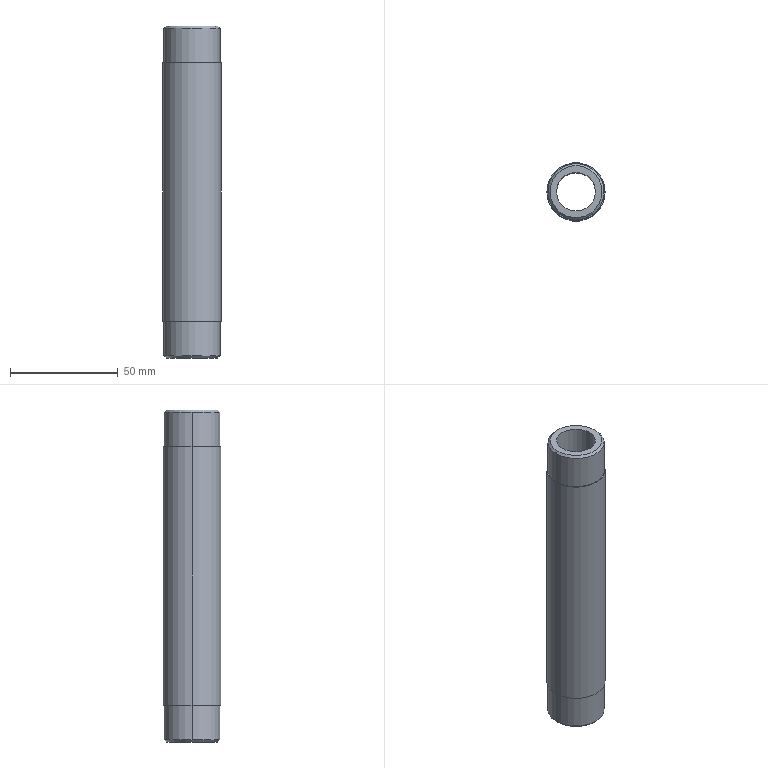Part | SolidWorks | features ICE 2, Chamfer 1, Extrusion 1, MirrorPattern 1 | 1 solid | 16 faces | box 27 x 27 x 154 mm | volume 47629 mm3 | cylinder 8 | cone 4 | plane 4 | commonest cylinder face diameters 26.1 x4 18 x2 27 x2
STEP:
#1=CARTESIAN_POINT('',(12.05,0.,77.));
#2=VERTEX_POINT('',#1);
#3=CARTESIAN_POINT('',(-12.05,0.,77.));
#4=VERTEX_POINT('',#3);
#5=CARTESIAN_POINT('',(0.,0.,77.));
#6=DIRECTION('',(0.,0.,1.));
#7=DIRECTION('',(1.,0.,0.));
#8=AXIS2_PLACEMENT_3D('',#5,#6,#7);
#9=CIRCLE('',#8,12.05);
#10=EDGE_CURVE('',#2,#4,#9,.T.);
#11=ORIENTED_EDGE('',*,*,#10,.F.);
#12=CARTESIAN_POINT('',(13.05,0.,76.));
#13=VERTEX_POINT('',#12);
#14=CARTESIAN_POINT('',(13.05,0.,76.));
#15=DIRECTION('',(0.7071,0.,-0.7071));
#16=VECTOR('',#15,1000.);
#17=LINE('',#14,#16);
#18=EDGE_CURVE('',#2,#13,#17,.T.);
#19=ORIENTED_EDGE('',*,*,#18,.T.);
#20=CARTESIAN_POINT('',(-13.05,0.,76.));
#21=VERTEX_POINT('',#20);
#22=CARTESIAN_POINT('',(0.,0.,76.));
#23=DIRECTION('',(0.,0.,-1.));
#24=DIRECTION('',(1.,0.,0.));
#25=AXIS2_PLACEMENT_3D('',#22,#23,#24);
#26=CIRCLE('',#25,13.05);
#27=EDGE_CURVE('',#21,#13,#26,.T.);
#28=ORIENTED_EDGE('',*,*,#27,.F.);
#29=CARTESIAN_POINT('',(-13.05,0.,76.));
#30=DIRECTION('',(-0.7071,0.,-0.7071));
#31=VECTOR('',#30,1000.);
#32=LINE('',#29,#31);
#33=EDGE_CURVE('',#4,#21,#32,.T.);
#34=ORIENTED_EDGE('',*,*,#33,.F.);
#35=EDGE_LOOP('',(#11,#19,#28,#34));
#36=FACE_OUTER_BOUND('',#35,.T.);
#37=CARTESIAN_POINT('',(0.,0.,76.));
#38=DIRECTION('',(0.,0.,-1.));
#39=DIRECTION('',(-1.,0.,0.));
#40=AXIS2_PLACEMENT_3D('',#37,#38,#39);
#41=CONICAL_SURFACE('',#40,13.05,0.7854);
#42=ADVANCED_FACE('',(#36),#41,.T.);
#43=CARTESIAN_POINT('',(-12.05,0.,-77.));
#44=VERTEX_POINT('',#43);
#45=CARTESIAN_POINT('',(12.05,0.,-77.));
#46=VERTEX_POINT('',#45);
#47=CARTESIAN_POINT('',(0.,0.,-77.));
#48=DIRECTION('',(0.,0.,-1.));
#49=DIRECTION('',(-1.,0.,0.));
#50=AXIS2_PLACEMENT_3D('',#47,#48,#49);
#51=CIRCLE('',#50,12.05);
#52=EDGE_CURVE('',#44,#46,#51,.T.);
#53=ORIENTED_EDGE('',*,*,#52,.F.);
#54=CARTESIAN_POINT('',(-13.05,0.,-76.));
#55=VERTEX_POINT('',#54);
#56=CARTESIAN_POINT('',(-12.05,0.,-77.));
#57=DIRECTION('',(-0.7071,0.,0.7071));
#58=VECTOR('',#57,1000.);
#59=LINE('',#56,#58);
#60=EDGE_CURVE('',#44,#55,#59,.T.);
#61=ORIENTED_EDGE('',*,*,#60,.T.);
#62=CARTESIAN_POINT('',(13.05,0.,-76.));
#63=VERTEX_POINT('',#62);
#64=CARTESIAN_POINT('',(0.,0.,-76.));
#65=DIRECTION('',(0.,0.,1.));
#66=DIRECTION('',(-1.,0.,0.));
#67=AXIS2_PLACEMENT_3D('',#64,#65,#66);
#68=CIRCLE('',#67,13.05);
#69=EDGE_CURVE('',#63,#55,#68,.T.);
#70=ORIENTED_EDGE('',*,*,#69,.F.);
#71=CARTESIAN_POINT('',(12.05,0.,-77.));
#72=DIRECTION('',(0.7071,0.,0.7071));
#73=VECTOR('',#72,1000.);
#74=LINE('',#71,#73);
#75=EDGE_CURVE('',#46,#63,#74,.T.);
#76=ORIENTED_EDGE('',*,*,#75,.F.);
#77=EDGE_LOOP('',(#53,#61,#70,#76));
#78=FACE_OUTER_BOUND('',#77,.T.);
#79=CARTESIAN_POINT('',(0.,0.,-77.));
#80=DIRECTION('',(0.,0.,1.));
#81=DIRECTION('',(1.,0.,0.));
#82=AXIS2_PLACEMENT_3D('',#79,#80,#81);
#83=CONICAL_SURFACE('',#82,12.05,0.7854);
#84=ADVANCED_FACE('',(#78),#83,.T.);
#85=CARTESIAN_POINT('',(9.,0.,77.));
#86=VERTEX_POINT('',#85);
#87=CARTESIAN_POINT('',(-9.,0.,77.));
#88=VERTEX_POINT('',#87);
#89=CARTESIAN_POINT('',(0.,0.,77.));
#90=DIRECTION('',(0.,0.,-1.));
#91=DIRECTION('',(1.,0.,0.));
#92=AXIS2_PLACEMENT_3D('',#89,#90,#91);
#93=CIRCLE('',#92,9.);
#94=EDGE_CURVE('',#86,#88,#93,.T.);
#95=ORIENTED_EDGE('',*,*,#94,.F.);
#96=CARTESIAN_POINT('',(9.,0.,-77.));
#97=VERTEX_POINT('',#96);
#98=CARTESIAN_POINT('',(9.,0.,77.001));
#99=DIRECTION('',(0.,0.,-1.));
#100=VECTOR('',#99,1000.);
#101=LINE('',#98,#100);
#102=EDGE_CURVE('',#86,#97,#101,.T.);
#103=ORIENTED_EDGE('',*,*,#102,.T.);
#104=CARTESIAN_POINT('',(-9.,0.,-77.));
#105=VERTEX_POINT('',#104);
#106=CARTESIAN_POINT('',(0.,0.,-77.));
#107=DIRECTION('',(0.,0.,-1.));
#108=DIRECTION('',(-1.,0.,0.));
#109=AXIS2_PLACEMENT_3D('',#106,#107,#108);
#110=CIRCLE('',#109,9.);
#111=EDGE_CURVE('',#97,#105,#110,.T.);
#112=ORIENTED_EDGE('',*,*,#111,.T.);
#113=CARTESIAN_POINT('',(-9.,0.,77.001));
#114=DIRECTION('',(0.,0.,-1.));
#115=VECTOR('',#114,1000.);
#116=LINE('',#113,#115);
#117=EDGE_CURVE('',#88,#105,#116,.T.);
#118=ORIENTED_EDGE('',*,*,#117,.F.);
#119=EDGE_LOOP('',(#95,#103,#112,#118));
#120=FACE_OUTER_BOUND('',#119,.T.);
#121=CARTESIAN_POINT('',(0.,0.,77.001));
#122=DIRECTION('',(0.,0.,-1.));
#123=DIRECTION('',(-1.,0.,0.));
#124=AXIS2_PLACEMENT_3D('',#121,#122,#123);
#125=CYLINDRICAL_SURFACE('',#124,9.);
#126=ADVANCED_FACE('',(#120),#125,.F.);
#127=ORIENTED_EDGE('',*,*,#27,.T.);
#128=CARTESIAN_POINT('',(13.05,0.,60.));
#129=VERTEX_POINT('',#128);
#130=CARTESIAN_POINT('',(13.05,0.,77.));
#131=DIRECTION('',(0.,0.,-1.));
#132=VECTOR('',#131,1000.);
#133=LINE('',#130,#132);
#134=EDGE_CURVE('',#13,#129,#133,.T.);
#135=ORIENTED_EDGE('',*,*,#134,.T.);
#136=CARTESIAN_POINT('',(-13.05,0.,60.));
#137=VERTEX_POINT('',#136);
#138=CARTESIAN_POINT('',(0.,0.,60.));
#139=DIRECTION('',(0.,0.,-1.));
#140=DIRECTION('',(-1.,0.,0.));
#141=AXIS2_PLACEMENT_3D('',#138,#139,#140);
#142=CIRCLE('',#141,13.05);
#143=EDGE_CURVE('',#137,#129,#142,.T.);
#144=ORIENTED_EDGE('',*,*,#143,.F.);
#145=CARTESIAN_POINT('',(-13.05,0.,77.));
#146=DIRECTION('',(0.,0.,-1.));
#147=VECTOR('',#146,1000.);
#148=LINE('',#145,#147);
#149=EDGE_CURVE('',#21,#137,#148,.T.);
#150=ORIENTED_EDGE('',*,*,#149,.F.);
#151=EDGE_LOOP('',(#127,#135,#144,#150));
#152=FACE_OUTER_BOUND('',#151,.T.);
#153=CARTESIAN_POINT('',(0.,0.,77.));
#154=DIRECTION('',(0.,0.,-1.));
#155=DIRECTION('',(-1.,0.,0.));
#156=AXIS2_PLACEMENT_3D('',#153,#154,#155);
#157=CYLINDRICAL_SURFACE('',#156,13.05);
#158=ADVANCED_FACE('',(#152),#157,.T.);
#159=ORIENTED_EDGE('',*,*,#69,.T.);
#160=CARTESIAN_POINT('',(-13.05,0.,-60.));
#161=VERTEX_POINT('',#160);
#162=CARTESIAN_POINT('',(-13.05,0.,-77.));
#163=DIRECTION('',(0.,0.,1.));
#164=VECTOR('',#163,1000.);
#165=LINE('',#162,#164);
#166=EDGE_CURVE('',#55,#161,#165,.T.);
#167=ORIENTED_EDGE('',*,*,#166,.T.);
#168=CARTESIAN_POINT('',(13.05,0.,-60.));
#169=VERTEX_POINT('',#168);
#170=CARTESIAN_POINT('',(0.,0.,-60.));
#171=DIRECTION('',(0.,0.,-1.));
#172=DIRECTION('',(-1.,0.,0.));
#173=AXIS2_PLACEMENT_3D('',#170,#171,#172);
#174=CIRCLE('',#173,13.05);
#175=EDGE_CURVE('',#161,#169,#174,.T.);
#176=ORIENTED_EDGE('',*,*,#175,.T.);
#177=CARTESIAN_POINT('',(13.05,0.,-77.));
#178=DIRECTION('',(0.,0.,1.));
#179=VECTOR('',#178,1000.);
#180=LINE('',#177,#179);
#181=EDGE_CURVE('',#63,#169,#180,.T.);
#182=ORIENTED_EDGE('',*,*,#181,.F.);
#183=EDGE_LOOP('',(#159,#167,#176,#182));
#184=FACE_OUTER_BOUND('',#183,.T.);
#185=CARTESIAN_POINT('',(0.,0.,-77.));
#186=DIRECTION('',(0.,0.,1.));
#187=DIRECTION('',(1.,0.,0.));
#188=AXIS2_PLACEMENT_3D('',#185,#186,#187);
#189=CYLINDRICAL_SURFACE('',#188,13.05);
#190=ADVANCED_FACE('',(#184),#189,.T.);
#191=CARTESIAN_POINT('',(13.5,0.,60.));
#192=VERTEX_POINT('',#191);
#193=CARTESIAN_POINT('',(-13.5,0.,60.));
#194=VERTEX_POINT('',#193);
#195=CARTESIAN_POINT('',(0.,0.,60.));
#196=DIRECTION('',(0.,0.,1.));
#197=DIRECTION('',(1.,0.,0.));
#198=AXIS2_PLACEMENT_3D('',#195,#196,#197);
#199=CIRCLE('',#198,13.5);
#200=EDGE_CURVE('',#192,#194,#199,.T.);
#201=ORIENTED_EDGE('',*,*,#200,.F.);
#202=CARTESIAN_POINT('',(13.5,0.,-60.));
#203=VERTEX_POINT('',#202);
#204=CARTESIAN_POINT('',(13.5,0.,60.));
#205=DIRECTION('',(0.,0.,-1.));
#206=VECTOR('',#205,1000.);
#207=LINE('',#204,#206);
#208=EDGE_CURVE('',#192,#203,#207,.T.);
#209=ORIENTED_EDGE('',*,*,#208,.T.);
#210=CARTESIAN_POINT('',(-13.5,0.,-60.));
#211=VERTEX_POINT('',#210);
#212=CARTESIAN_POINT('',(0.,0.,-60.));
#213=DIRECTION('',(0.,0.,1.));
#214=DIRECTION('',(1.,0.,0.));
#215=AXIS2_PLACEMENT_3D('',#212,#213,#214);
#216=CIRCLE('',#215,13.5);
#217=EDGE_CURVE('',#203,#211,#216,.T.);
#218=ORIENTED_EDGE('',*,*,#217,.T.);
#219=CARTESIAN_POINT('',(-13.5,0.,60.));
#220=DIRECTION('',(0.,0.,-1.));
#221=VECTOR('',#220,1000.);
#222=LINE('',#219,#221);
#223=EDGE_CURVE('',#194,#211,#222,.T.);
#224=ORIENTED_EDGE('',*,*,#223,.F.);
#225=EDGE_LOOP('',(#201,#209,#218,#224));
#226=FACE_OUTER_BOUND('',#225,.T.);
#227=CARTESIAN_POINT('',(0.,0.,60.));
#228=DIRECTION('',(0.,0.,-1.));
#229=DIRECTION('',(-1.,0.,0.));
#230=AXIS2_PLACEMENT_3D('',#227,#228,#229);
#231=CYLINDRICAL_SURFACE('',#230,13.5);
#232=ADVANCED_FACE('',(#226),#231,.T.);
#233=ORIENTED_EDGE('',*,*,#208,.F.);
#234=CARTESIAN_POINT('',(0.,0.,60.));
#235=DIRECTION('',(0.,0.,1.));
#236=DIRECTION('',(1.,0.,0.));
#237=AXIS2_PLACEMENT_3D('',#234,#235,#236);
#238=CIRCLE('',#237,13.5);
#239=EDGE_CURVE('',#194,#192,#238,.T.);
#240=ORIENTED_EDGE('',*,*,#239,.F.);
#241=ORIENTED_EDGE('',*,*,#223,.T.);
#242=CARTESIAN_POINT('',(0.,0.,-60.));
#243=DIRECTION('',(0.,0.,1.));
#244=DIRECTION('',(1.,0.,0.));
#245=AXIS2_PLACEMENT_3D('',#242,#243,#244);
#246=CIRCLE('',#245,13.5);
#247=EDGE_CURVE('',#211,#203,#246,.T.);
#248=ORIENTED_EDGE('',*,*,#247,.T.);
#249=EDGE_LOOP('',(#233,#240,#241,#248));
#250=FACE_OUTER_BOUND('',#249,.T.);
#251=CARTESIAN_POINT('',(0.,0.,60.));
#252=DIRECTION('',(0.,0.,-1.));
#253=DIRECTION('',(-1.,0.,0.));
#254=AXIS2_PLACEMENT_3D('',#251,#252,#253);
#255=CYLINDRICAL_SURFACE('',#254,13.5);
#256=ADVANCED_FACE('',(#250),#255,.T.);
#257=ORIENTED_EDGE('',*,*,#143,.T.);
#258=CARTESIAN_POINT('',(0.,0.,60.));
#259=DIRECTION('',(0.,0.,-1.));
#260=DIRECTION('',(-1.,0.,0.));
#261=AXIS2_PLACEMENT_3D('',#258,#259,#260);
#262=CIRCLE('',#261,13.05);
#263=EDGE_CURVE('',#129,#137,#262,.T.);
#264=ORIENTED_EDGE('',*,*,#263,.T.);
#265=EDGE_LOOP('',(#257,#264));
#266=FACE_BOUND('',#265,.T.);
#267=ORIENTED_EDGE('',*,*,#239,.T.);
#268=ORIENTED_EDGE('',*,*,#200,.T.);
#269=EDGE_LOOP('',(#267,#268));
#270=FACE_OUTER_BOUND('',#269,.T.);
#271=CARTESIAN_POINT('',(0.,0.,60.));
#272=DIRECTION('',(0.,0.,1.));
#273=DIRECTION('',(1.,0.,0.));
#274=AXIS2_PLACEMENT_3D('',#271,#272,#273);
#275=PLANE('',#274);
#276=ADVANCED_FACE('',(#266,#270),#275,.T.);
#277=CARTESIAN_POINT('',(0.,0.,-60.));
#278=DIRECTION('',(0.,0.,-1.));
#279=DIRECTION('',(-1.,0.,0.));
#280=AXIS2_PLACEMENT_3D('',#277,#278,#279);
#281=CIRCLE('',#280,13.05);
#282=EDGE_CURVE('',#169,#161,#281,.T.);
#283=ORIENTED_EDGE('',*,*,#282,.F.);
#284=ORIENTED_EDGE('',*,*,#175,.F.);
#285=EDGE_LOOP('',(#283,#284));
#286=FACE_BOUND('',#285,.T.);
#287=ORIENTED_EDGE('',*,*,#247,.F.);
#288=ORIENTED_EDGE('',*,*,#217,.F.);
#289=EDGE_LOOP('',(#287,#288));
#290=FACE_OUTER_BOUND('',#289,.T.);
#291=CARTESIAN_POINT('',(0.,0.,-60.));
#292=DIRECTION('',(0.,0.,1.));
#293=DIRECTION('',(1.,0.,0.));
#294=AXIS2_PLACEMENT_3D('',#291,#292,#293);
#295=PLANE('',#294);
#296=ADVANCED_FACE('',(#286,#290),#295,.F.);
#297=ORIENTED_EDGE('',*,*,#166,.F.);
#298=CARTESIAN_POINT('',(0.,0.,-76.));
#299=DIRECTION('',(0.,0.,1.));
#300=DIRECTION('',(-1.,0.,0.));
#301=AXIS2_PLACEMENT_3D('',#298,#299,#300);
#302=CIRCLE('',#301,13.05);
#303=EDGE_CURVE('',#55,#63,#302,.T.);
#304=ORIENTED_EDGE('',*,*,#303,.T.);
#305=ORIENTED_EDGE('',*,*,#181,.T.);
#306=ORIENTED_EDGE('',*,*,#282,.T.);
#307=EDGE_LOOP('',(#297,#304,#305,#306));
#308=FACE_OUTER_BOUND('',#307,.T.);
#309=CARTESIAN_POINT('',(0.,0.,-77.));
#310=DIRECTION('',(0.,0.,1.));
#311=DIRECTION('',(1.,0.,0.));
#312=AXIS2_PLACEMENT_3D('',#309,#310,#311);
#313=CYLINDRICAL_SURFACE('',#312,13.05);
#314=ADVANCED_FACE('',(#308),#313,.T.);
#315=CARTESIAN_POINT('',(0.,0.,-77.));
#316=DIRECTION('',(0.,0.,-1.));
#317=DIRECTION('',(-1.,0.,0.));
#318=AXIS2_PLACEMENT_3D('',#315,#316,#317);
#319=CIRCLE('',#318,12.05);
#320=EDGE_CURVE('',#46,#44,#319,.T.);
#321=ORIENTED_EDGE('',*,*,#320,.T.);
#322=ORIENTED_EDGE('',*,*,#52,.T.);
#323=EDGE_LOOP('',(#321,#322));
#324=FACE_OUTER_BOUND('',#323,.T.);
#325=CARTESIAN_POINT('',(0.,0.,-77.));
#326=DIRECTION('',(0.,0.,-1.));
#327=DIRECTION('',(-1.,0.,0.));
#328=AXIS2_PLACEMENT_3D('',#325,#326,#327);
#329=CIRCLE('',#328,9.);
#330=EDGE_CURVE('',#105,#97,#329,.T.);
#331=ORIENTED_EDGE('',*,*,#330,.F.);
#332=ORIENTED_EDGE('',*,*,#111,.F.);
#333=EDGE_LOOP('',(#331,#332));
#334=FACE_BOUND('',#333,.T.);
#335=CARTESIAN_POINT('',(0.,0.,-77.));
#336=DIRECTION('',(0.,0.,-1.));
#337=DIRECTION('',(-1.,0.,0.));
#338=AXIS2_PLACEMENT_3D('',#335,#336,#337);
#339=PLANE('',#338);
#340=ADVANCED_FACE('',(#324,#334),#339,.T.);
#341=ORIENTED_EDGE('',*,*,#134,.F.);
#342=CARTESIAN_POINT('',(0.,0.,76.));
#343=DIRECTION('',(0.,0.,-1.));
#344=DIRECTION('',(1.,0.,0.));
#345=AXIS2_PLACEMENT_3D('',#342,#343,#344);
#346=CIRCLE('',#345,13.05);
#347=EDGE_CURVE('',#13,#21,#346,.T.);
#348=ORIENTED_EDGE('',*,*,#347,.T.);
#349=ORIENTED_EDGE('',*,*,#149,.T.);
#350=ORIENTED_EDGE('',*,*,#263,.F.);
#351=EDGE_LOOP('',(#341,#348,#349,#350));
#352=FACE_OUTER_BOUND('',#351,.T.);
#353=CARTESIAN_POINT('',(0.,0.,77.));
#354=DIRECTION('',(0.,0.,-1.));
#355=DIRECTION('',(-1.,0.,0.));
#356=AXIS2_PLACEMENT_3D('',#353,#354,#355);
#357=CYLINDRICAL_SURFACE('',#356,13.05);
#358=ADVANCED_FACE('',(#352),#357,.T.);
#359=CARTESIAN_POINT('',(0.,0.,77.));
#360=DIRECTION('',(0.,0.,1.));
#361=DIRECTION('',(1.,0.,0.));
#362=AXIS2_PLACEMENT_3D('',#359,#360,#361);
#363=CIRCLE('',#362,12.05);
#364=EDGE_CURVE('',#4,#2,#363,.T.);
#365=ORIENTED_EDGE('',*,*,#364,.T.);
#366=ORIENTED_EDGE('',*,*,#10,.T.);
#367=EDGE_LOOP('',(#365,#366));
#368=FACE_OUTER_BOUND('',#367,.T.);
#369=CARTESIAN_POINT('',(0.,0.,77.));
#370=DIRECTION('',(0.,0.,-1.));
#371=DIRECTION('',(1.,0.,0.));
#372=AXIS2_PLACEMENT_3D('',#369,#370,#371);
#373=CIRCLE('',#372,9.);
#374=EDGE_CURVE('',#88,#86,#373,.T.);
#375=ORIENTED_EDGE('',*,*,#374,.T.);
#376=ORIENTED_EDGE('',*,*,#94,.T.);
#377=EDGE_LOOP('',(#375,#376));
#378=FACE_BOUND('',#377,.T.);
#379=CARTESIAN_POINT('',(0.,0.,77.));
#380=DIRECTION('',(0.,0.,1.));
#381=DIRECTION('',(-1.,0.,0.));
#382=AXIS2_PLACEMENT_3D('',#379,#380,#381);
#383=PLANE('',#382);
#384=ADVANCED_FACE('',(#368,#378),#383,.T.);
#385=ORIENTED_EDGE('',*,*,#102,.F.);
#386=ORIENTED_EDGE('',*,*,#374,.F.);
#387=ORIENTED_EDGE('',*,*,#117,.T.);
#388=ORIENTED_EDGE('',*,*,#330,.T.);
#389=EDGE_LOOP('',(#385,#386,#387,#388));
#390=FACE_OUTER_BOUND('',#389,.T.);
#391=CARTESIAN_POINT('',(0.,0.,77.001));
#392=DIRECTION('',(0.,0.,-1.));
#393=DIRECTION('',(-1.,0.,0.));
#394=AXIS2_PLACEMENT_3D('',#391,#392,#393);
#395=CYLINDRICAL_SURFACE('',#394,9.);
#396=ADVANCED_FACE('',(#390),#395,.F.);
#397=ORIENTED_EDGE('',*,*,#60,.F.);
#398=ORIENTED_EDGE('',*,*,#320,.F.);
#399=ORIENTED_EDGE('',*,*,#75,.T.);
#400=ORIENTED_EDGE('',*,*,#303,.F.);
#401=EDGE_LOOP('',(#397,#398,#399,#400));
#402=FACE_OUTER_BOUND('',#401,.T.);
#403=CARTESIAN_POINT('',(0.,0.,-77.));
#404=DIRECTION('',(0.,0.,1.));
#405=DIRECTION('',(1.,0.,0.));
#406=AXIS2_PLACEMENT_3D('',#403,#404,#405);
#407=CONICAL_SURFACE('',#406,12.05,0.7854);
#408=ADVANCED_FACE('',(#402),#407,.T.);
#409=ORIENTED_EDGE('',*,*,#18,.F.);
#410=ORIENTED_EDGE('',*,*,#364,.F.);
#411=ORIENTED_EDGE('',*,*,#33,.T.);
#412=ORIENTED_EDGE('',*,*,#347,.F.);
#413=EDGE_LOOP('',(#409,#410,#411,#412));
#414=FACE_OUTER_BOUND('',#413,.T.);
#415=CARTESIAN_POINT('',(0.,0.,76.));
#416=DIRECTION('',(0.,0.,-1.));
#417=DIRECTION('',(-1.,0.,0.));
#418=AXIS2_PLACEMENT_3D('',#415,#416,#417);
#419=CONICAL_SURFACE('',#418,13.05,0.7854);
#420=ADVANCED_FACE('',(#414),#419,.T.);
#421=CLOSED_SHELL('',(#42,#84,#126,#158,#190,#232,#256,#276,#296,#314,#340,#358,#384,#396,#408,#420));
#422=MANIFOLD_SOLID_BREP('',#421);
#423=CARTESIAN_POINT('',(0.,0.,0.));
#424=DIRECTION('',(0.,0.,1.));
#425=DIRECTION('',(1.,0.,0.));
#426=AXIS2_PLACEMENT_3D('',#423,#424,#425);
#427=(LENGTH_UNIT()NAMED_UNIT(*)SI_UNIT(.MILLI.,.METRE.));
#428=UNCERTAINTY_MEASURE_WITH_UNIT(LENGTH_MEASURE(0.00001),#427,'','');
#429=(NAMED_UNIT(*)PLANE_ANGLE_UNIT()SI_UNIT($,.RADIAN.));
#430=(NAMED_UNIT(*)SI_UNIT($,.STERADIAN.)SOLID_ANGLE_UNIT());
#431=(GEOMETRIC_REPRESENTATION_CONTEXT(3)GLOBAL_UNCERTAINTY_ASSIGNED_CONTEXT((#428))GLOBAL_UNIT_ASSIGNED_CONTEXT((#427,#429,#430))REPRESENTATION_CONTEXT('',''));
#432=ADVANCED_BREP_SHAPE_REPRESENTATION('',(#422,#426),#431);